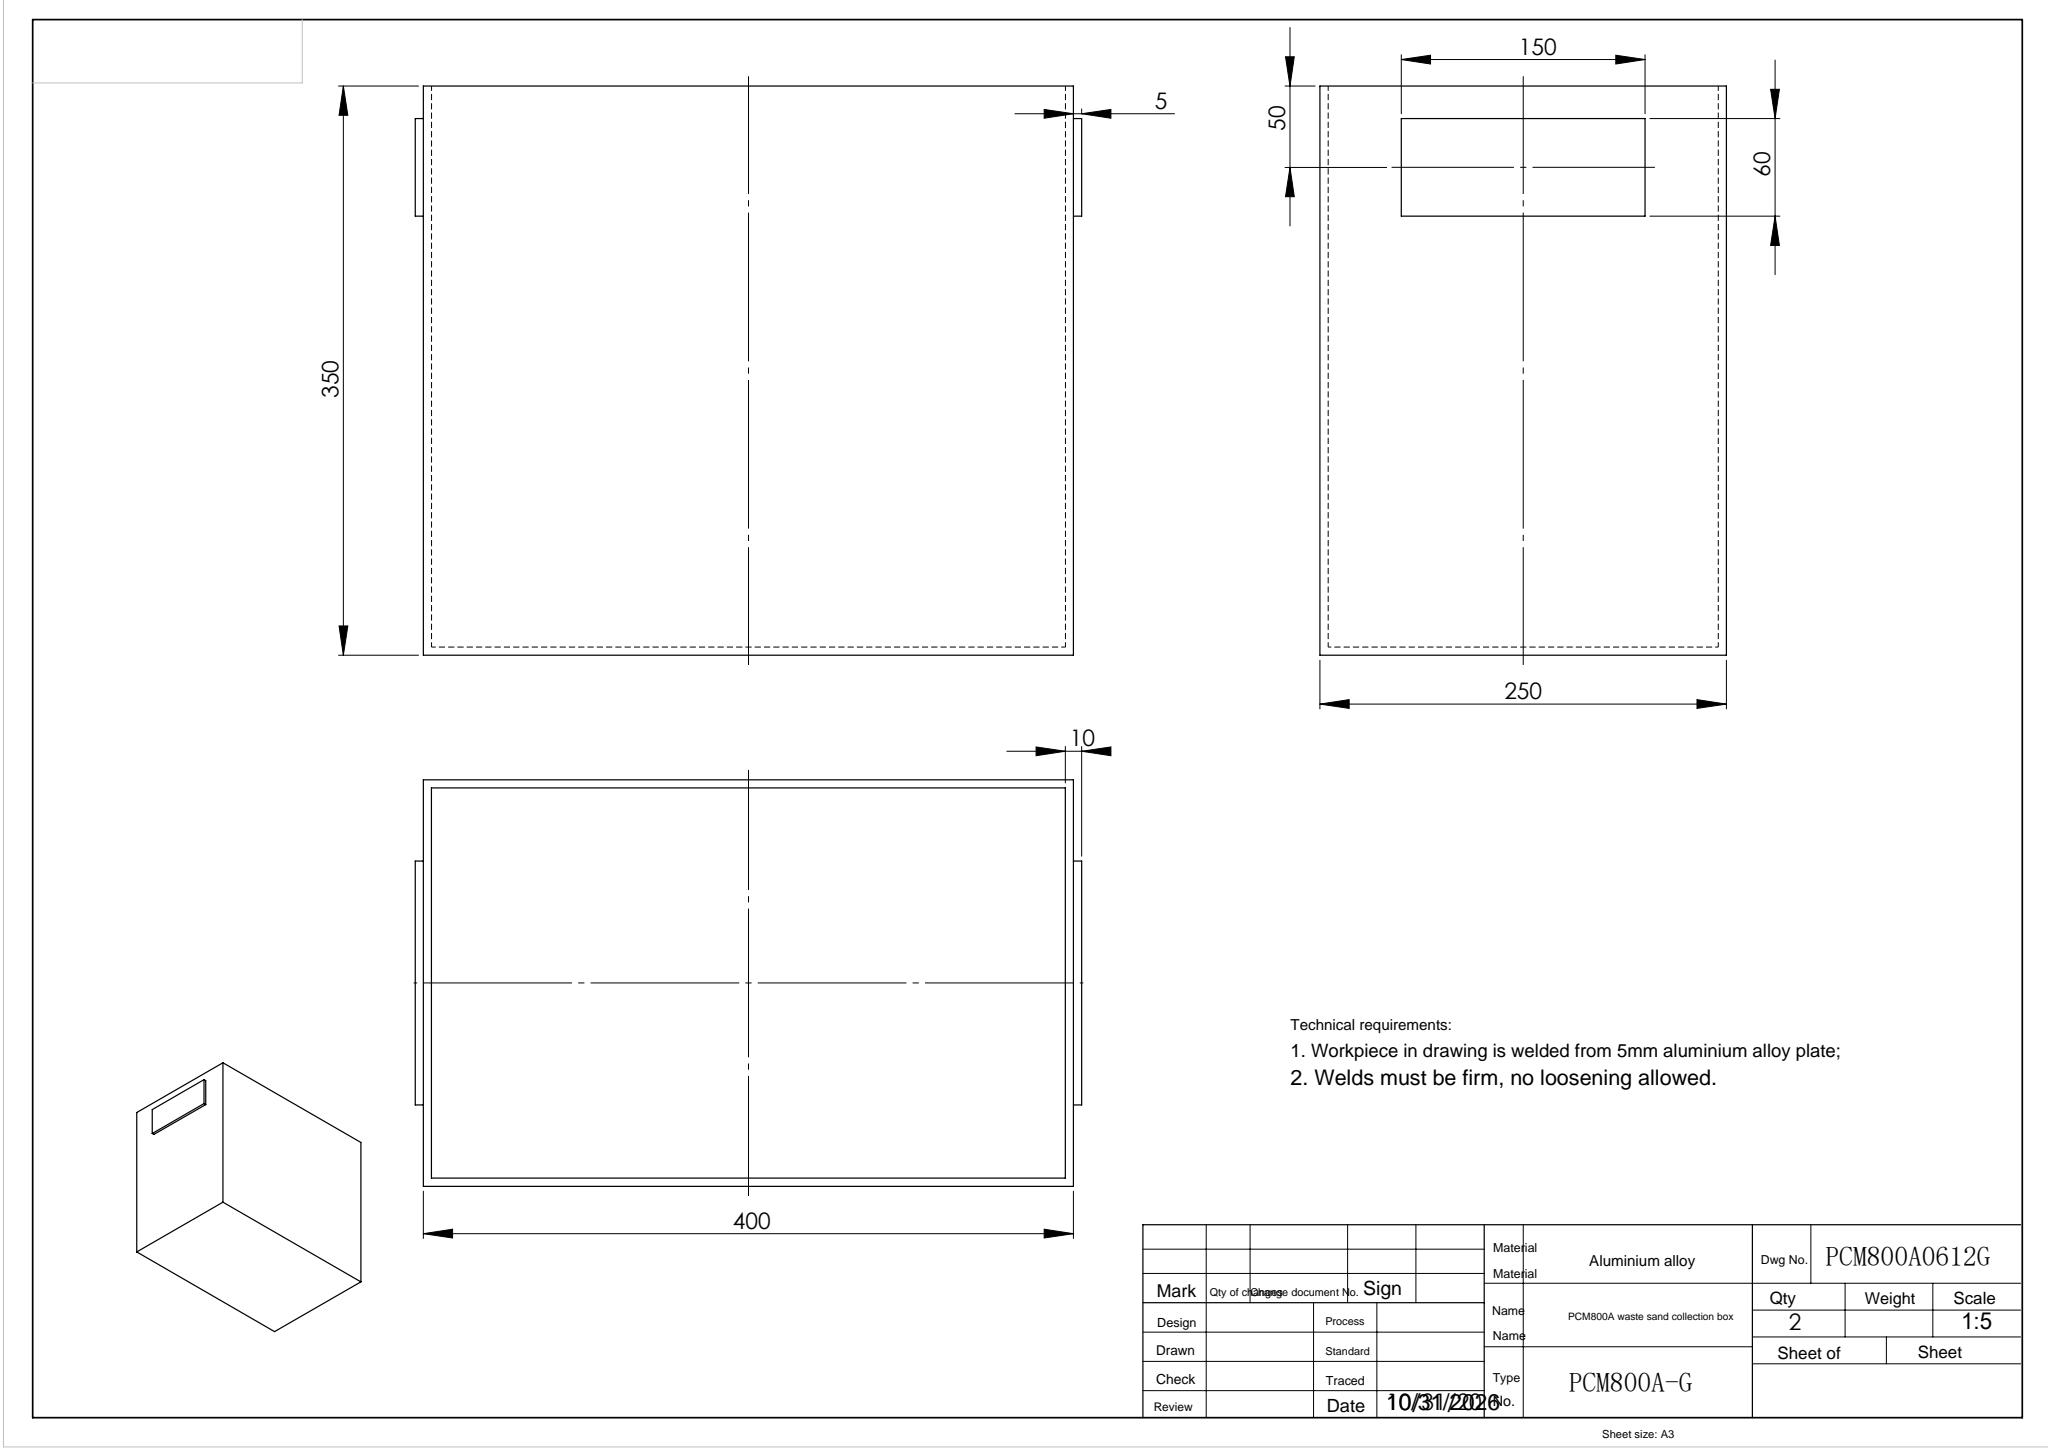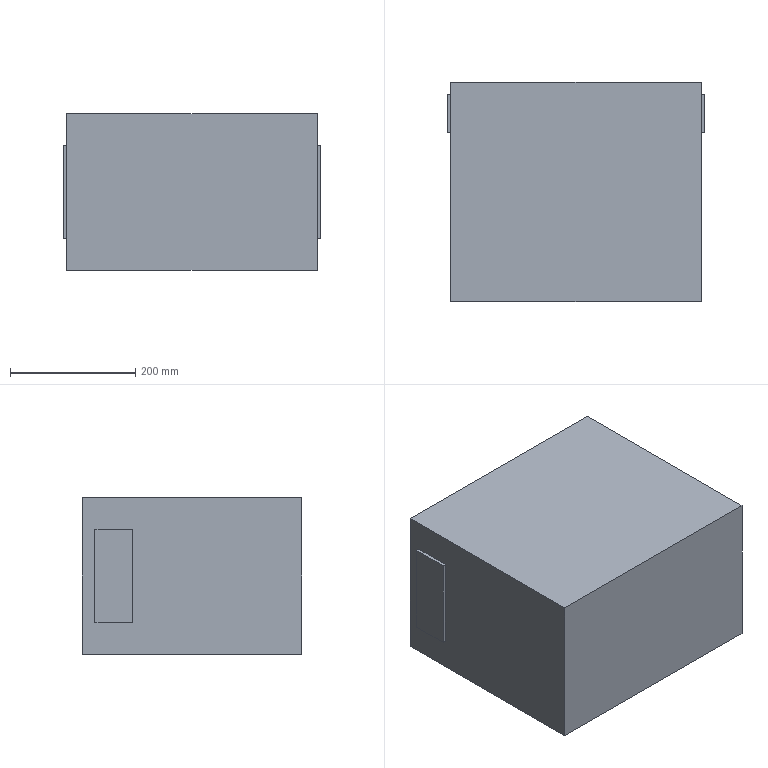Part | SolidWorks | features ICE 2, Extrusion 1, Shell 1 | 1 solid | 21 faces | box 410 x 350 x 250 mm | volume 2798000 mm3 | plane 21
STEP:
#1=CARTESIAN_POINT('',(0.,0.,-250.));
#2=VERTEX_POINT('',#1);
#3=CARTESIAN_POINT('',(0.,0.,0.));
#4=VERTEX_POINT('',#3);
#5=CARTESIAN_POINT('',(0.,0.,0.));
#6=DIRECTION('',(0.,0.,1.));
#7=VECTOR('',#6,1000.);
#8=LINE('',#5,#7);
#9=EDGE_CURVE('',#2,#4,#8,.T.);
#10=ORIENTED_EDGE('',*,*,#9,.T.);
#11=CARTESIAN_POINT('',(0.,350.,0.));
#12=VERTEX_POINT('',#11);
#13=CARTESIAN_POINT('',(0.,350.,0.));
#14=DIRECTION('',(0.,-1.,0.));
#15=VECTOR('',#14,1000.);
#16=LINE('',#13,#15);
#17=EDGE_CURVE('',#12,#4,#16,.T.);
#18=ORIENTED_EDGE('',*,*,#17,.F.);
#19=CARTESIAN_POINT('',(0.,350.,-250.));
#20=VERTEX_POINT('',#19);
#21=CARTESIAN_POINT('',(0.,350.,0.));
#22=DIRECTION('',(0.,0.,1.));
#23=VECTOR('',#22,1000.);
#24=LINE('',#21,#23);
#25=EDGE_CURVE('',#20,#12,#24,.T.);
#26=ORIENTED_EDGE('',*,*,#25,.F.);
#27=CARTESIAN_POINT('',(0.,350.,-250.));
#28=DIRECTION('',(0.,-1.,0.));
#29=VECTOR('',#28,1000.);
#30=LINE('',#27,#29);
#31=EDGE_CURVE('',#20,#2,#30,.T.);
#32=ORIENTED_EDGE('',*,*,#31,.T.);
#33=EDGE_LOOP('',(#10,#18,#26,#32));
#34=FACE_OUTER_BOUND('',#33,.T.);
#35=CARTESIAN_POINT('',(0.,330.,-200.));
#36=VERTEX_POINT('',#35);
#37=CARTESIAN_POINT('',(0.,270.,-200.));
#38=VERTEX_POINT('',#37);
#39=CARTESIAN_POINT('',(0.,330.,-200.));
#40=DIRECTION('',(0.,-1.,0.));
#41=VECTOR('',#40,1000.);
#42=LINE('',#39,#41);
#43=EDGE_CURVE('',#36,#38,#42,.T.);
#44=ORIENTED_EDGE('',*,*,#43,.F.);
#45=CARTESIAN_POINT('',(0.,330.,-50.));
#46=VERTEX_POINT('',#45);
#47=CARTESIAN_POINT('',(0.,330.,-200.));
#48=DIRECTION('',(0.,0.,-1.));
#49=VECTOR('',#48,1000.);
#50=LINE('',#47,#49);
#51=EDGE_CURVE('',#46,#36,#50,.T.);
#52=ORIENTED_EDGE('',*,*,#51,.F.);
#53=CARTESIAN_POINT('',(0.,270.,-50.));
#54=VERTEX_POINT('',#53);
#55=CARTESIAN_POINT('',(0.,330.,-50.));
#56=DIRECTION('',(0.,1.,0.));
#57=VECTOR('',#56,1000.);
#58=LINE('',#55,#57);
#59=EDGE_CURVE('',#54,#46,#58,.T.);
#60=ORIENTED_EDGE('',*,*,#59,.F.);
#61=CARTESIAN_POINT('',(0.,270.,-200.));
#62=DIRECTION('',(0.,0.,1.));
#63=VECTOR('',#62,1000.);
#64=LINE('',#61,#63);
#65=EDGE_CURVE('',#38,#54,#64,.T.);
#66=ORIENTED_EDGE('',*,*,#65,.F.);
#67=EDGE_LOOP('',(#44,#52,#60,#66));
#68=FACE_BOUND('',#67,.T.);
#69=CARTESIAN_POINT('',(0.,350.,0.));
#70=DIRECTION('',(1.,0.,0.));
#71=DIRECTION('',(0.,0.,-1.));
#72=AXIS2_PLACEMENT_3D('',#69,#70,#71);
#73=PLANE('',#72);
#74=ADVANCED_FACE('',(#34,#68),#73,.F.);
#75=CARTESIAN_POINT('',(400.,0.,0.));
#76=VERTEX_POINT('',#75);
#77=CARTESIAN_POINT('',(400.,0.,-250.));
#78=VERTEX_POINT('',#77);
#79=CARTESIAN_POINT('',(400.,0.,0.));
#80=DIRECTION('',(0.,0.,-1.));
#81=VECTOR('',#80,1000.);
#82=LINE('',#79,#81);
#83=EDGE_CURVE('',#76,#78,#82,.T.);
#84=ORIENTED_EDGE('',*,*,#83,.T.);
#85=CARTESIAN_POINT('',(400.,350.,-250.));
#86=VERTEX_POINT('',#85);
#87=CARTESIAN_POINT('',(400.,350.,-250.));
#88=DIRECTION('',(0.,-1.,0.));
#89=VECTOR('',#88,1000.);
#90=LINE('',#87,#89);
#91=EDGE_CURVE('',#86,#78,#90,.T.);
#92=ORIENTED_EDGE('',*,*,#91,.F.);
#93=CARTESIAN_POINT('',(400.,350.,0.));
#94=VERTEX_POINT('',#93);
#95=CARTESIAN_POINT('',(400.,350.,0.));
#96=DIRECTION('',(0.,0.,-1.));
#97=VECTOR('',#96,1000.);
#98=LINE('',#95,#97);
#99=EDGE_CURVE('',#94,#86,#98,.T.);
#100=ORIENTED_EDGE('',*,*,#99,.F.);
#101=CARTESIAN_POINT('',(400.,350.,0.));
#102=DIRECTION('',(0.,-1.,0.));
#103=VECTOR('',#102,1000.);
#104=LINE('',#101,#103);
#105=EDGE_CURVE('',#94,#76,#104,.T.);
#106=ORIENTED_EDGE('',*,*,#105,.T.);
#107=EDGE_LOOP('',(#84,#92,#100,#106));
#108=FACE_OUTER_BOUND('',#107,.T.);
#109=CARTESIAN_POINT('',(400.,330.,-50.));
#110=VERTEX_POINT('',#109);
#111=CARTESIAN_POINT('',(400.,270.,-50.));
#112=VERTEX_POINT('',#111);
#113=CARTESIAN_POINT('',(400.,330.,-50.));
#114=DIRECTION('',(0.,-1.,0.));
#115=VECTOR('',#114,1000.);
#116=LINE('',#113,#115);
#117=EDGE_CURVE('',#110,#112,#116,.T.);
#118=ORIENTED_EDGE('',*,*,#117,.F.);
#119=CARTESIAN_POINT('',(400.,330.,-200.));
#120=VERTEX_POINT('',#119);
#121=CARTESIAN_POINT('',(400.,330.,-50.));
#122=DIRECTION('',(0.,0.,1.));
#123=VECTOR('',#122,1000.);
#124=LINE('',#121,#123);
#125=EDGE_CURVE('',#120,#110,#124,.T.);
#126=ORIENTED_EDGE('',*,*,#125,.F.);
#127=CARTESIAN_POINT('',(400.,270.,-200.));
#128=VERTEX_POINT('',#127);
#129=CARTESIAN_POINT('',(400.,330.,-200.));
#130=DIRECTION('',(0.,1.,0.));
#131=VECTOR('',#130,1000.);
#132=LINE('',#129,#131);
#133=EDGE_CURVE('',#128,#120,#132,.T.);
#134=ORIENTED_EDGE('',*,*,#133,.F.);
#135=CARTESIAN_POINT('',(400.,270.,-50.));
#136=DIRECTION('',(0.,0.,-1.));
#137=VECTOR('',#136,1000.);
#138=LINE('',#135,#137);
#139=EDGE_CURVE('',#112,#128,#138,.T.);
#140=ORIENTED_EDGE('',*,*,#139,.F.);
#141=EDGE_LOOP('',(#118,#126,#134,#140));
#142=FACE_BOUND('',#141,.T.);
#143=CARTESIAN_POINT('',(400.,350.,0.));
#144=DIRECTION('',(-1.,0.,0.));
#145=DIRECTION('',(0.,0.,1.));
#146=AXIS2_PLACEMENT_3D('',#143,#144,#145);
#147=PLANE('',#146);
#148=ADVANCED_FACE('',(#108,#142),#147,.F.);
#149=ORIENTED_EDGE('',*,*,#25,.T.);
#150=CARTESIAN_POINT('',(0.,350.,0.));
#151=DIRECTION('',(1.,0.,0.));
#152=VECTOR('',#151,1000.);
#153=LINE('',#150,#152);
#154=EDGE_CURVE('',#12,#94,#153,.T.);
#155=ORIENTED_EDGE('',*,*,#154,.T.);
#156=ORIENTED_EDGE('',*,*,#99,.T.);
#157=CARTESIAN_POINT('',(0.,350.,-250.));
#158=DIRECTION('',(-1.,0.,0.));
#159=VECTOR('',#158,1000.);
#160=LINE('',#157,#159);
#161=EDGE_CURVE('',#86,#20,#160,.T.);
#162=ORIENTED_EDGE('',*,*,#161,.T.);
#163=EDGE_LOOP('',(#149,#155,#156,#162));
#164=FACE_OUTER_BOUND('',#163,.T.);
#165=CARTESIAN_POINT('',(5.,350.,-245.));
#166=VERTEX_POINT('',#165);
#167=CARTESIAN_POINT('',(5.,350.,-5.));
#168=VERTEX_POINT('',#167);
#169=CARTESIAN_POINT('',(5.,350.,-250.));
#170=DIRECTION('',(0.,0.,1.));
#171=VECTOR('',#170,1000.);
#172=LINE('',#169,#171);
#173=EDGE_CURVE('',#166,#168,#172,.T.);
#174=ORIENTED_EDGE('',*,*,#173,.F.);
#175=CARTESIAN_POINT('',(395.,350.,-245.));
#176=VERTEX_POINT('',#175);
#177=CARTESIAN_POINT('',(0.,350.,-245.));
#178=DIRECTION('',(-1.,0.,0.));
#179=VECTOR('',#178,1000.);
#180=LINE('',#177,#179);
#181=EDGE_CURVE('',#176,#166,#180,.T.);
#182=ORIENTED_EDGE('',*,*,#181,.F.);
#183=CARTESIAN_POINT('',(395.,350.,-5.));
#184=VERTEX_POINT('',#183);
#185=CARTESIAN_POINT('',(395.,350.,-250.));
#186=DIRECTION('',(0.,0.,-1.));
#187=VECTOR('',#186,1000.);
#188=LINE('',#185,#187);
#189=EDGE_CURVE('',#184,#176,#188,.T.);
#190=ORIENTED_EDGE('',*,*,#189,.F.);
#191=CARTESIAN_POINT('',(0.,350.,-5.));
#192=DIRECTION('',(1.,0.,0.));
#193=VECTOR('',#192,1000.);
#194=LINE('',#191,#193);
#195=EDGE_CURVE('',#168,#184,#194,.T.);
#196=ORIENTED_EDGE('',*,*,#195,.F.);
#197=EDGE_LOOP('',(#174,#182,#190,#196));
#198=FACE_BOUND('',#197,.T.);
#199=CARTESIAN_POINT('',(0.,350.,-250.));
#200=DIRECTION('',(0.,-1.,0.));
#201=DIRECTION('',(0.,0.,-1.));
#202=AXIS2_PLACEMENT_3D('',#199,#200,#201);
#203=PLANE('',#202);
#204=ADVANCED_FACE('',(#164,#198),#203,.F.);
#205=CARTESIAN_POINT('',(0.,0.,0.));
#206=DIRECTION('',(1.,0.,0.));
#207=VECTOR('',#206,1000.);
#208=LINE('',#205,#207);
#209=EDGE_CURVE('',#4,#76,#208,.T.);
#210=ORIENTED_EDGE('',*,*,#209,.T.);
#211=ORIENTED_EDGE('',*,*,#105,.F.);
#212=ORIENTED_EDGE('',*,*,#154,.F.);
#213=ORIENTED_EDGE('',*,*,#17,.T.);
#214=EDGE_LOOP('',(#210,#211,#212,#213));
#215=FACE_OUTER_BOUND('',#214,.T.);
#216=CARTESIAN_POINT('',(0.,350.,0.));
#217=DIRECTION('',(0.,0.,-1.));
#218=DIRECTION('',(-1.,0.,0.));
#219=AXIS2_PLACEMENT_3D('',#216,#217,#218);
#220=PLANE('',#219);
#221=ADVANCED_FACE('',(#215),#220,.F.);
#222=CARTESIAN_POINT('',(0.,0.,-250.));
#223=DIRECTION('',(-1.,0.,0.));
#224=VECTOR('',#223,1000.);
#225=LINE('',#222,#224);
#226=EDGE_CURVE('',#78,#2,#225,.T.);
#227=ORIENTED_EDGE('',*,*,#226,.T.);
#228=ORIENTED_EDGE('',*,*,#31,.F.);
#229=ORIENTED_EDGE('',*,*,#161,.F.);
#230=ORIENTED_EDGE('',*,*,#91,.T.);
#231=EDGE_LOOP('',(#227,#228,#229,#230));
#232=FACE_OUTER_BOUND('',#231,.T.);
#233=CARTESIAN_POINT('',(0.,350.,-250.));
#234=DIRECTION('',(0.,0.,1.));
#235=DIRECTION('',(1.,0.,0.));
#236=AXIS2_PLACEMENT_3D('',#233,#234,#235);
#237=PLANE('',#236);
#238=ADVANCED_FACE('',(#232),#237,.F.);
#239=ORIENTED_EDGE('',*,*,#9,.F.);
#240=ORIENTED_EDGE('',*,*,#226,.F.);
#241=ORIENTED_EDGE('',*,*,#83,.F.);
#242=ORIENTED_EDGE('',*,*,#209,.F.);
#243=EDGE_LOOP('',(#239,#240,#241,#242));
#244=FACE_OUTER_BOUND('',#243,.T.);
#245=CARTESIAN_POINT('',(0.,0.,-250.));
#246=DIRECTION('',(0.,-1.,0.));
#247=DIRECTION('',(0.,0.,-1.));
#248=AXIS2_PLACEMENT_3D('',#245,#246,#247);
#249=PLANE('',#248);
#250=ADVANCED_FACE('',(#244),#249,.T.);
#251=CARTESIAN_POINT('',(5.,5.,-245.));
#252=VERTEX_POINT('',#251);
#253=CARTESIAN_POINT('',(5.,5.,-5.));
#254=VERTEX_POINT('',#253);
#255=CARTESIAN_POINT('',(5.,5.,-250.));
#256=DIRECTION('',(0.,0.,1.));
#257=VECTOR('',#256,1000.);
#258=LINE('',#255,#257);
#259=EDGE_CURVE('',#252,#254,#258,.T.);
#260=ORIENTED_EDGE('',*,*,#259,.F.);
#261=CARTESIAN_POINT('',(5.,350.,-245.));
#262=DIRECTION('',(0.,-1.,0.));
#263=VECTOR('',#262,1000.);
#264=LINE('',#261,#263);
#265=EDGE_CURVE('',#166,#252,#264,.T.);
#266=ORIENTED_EDGE('',*,*,#265,.F.);
#267=ORIENTED_EDGE('',*,*,#173,.T.);
#268=CARTESIAN_POINT('',(5.,350.,-5.));
#269=DIRECTION('',(0.,-1.,0.));
#270=VECTOR('',#269,1000.);
#271=LINE('',#268,#270);
#272=EDGE_CURVE('',#168,#254,#271,.T.);
#273=ORIENTED_EDGE('',*,*,#272,.T.);
#274=EDGE_LOOP('',(#260,#266,#267,#273));
#275=FACE_OUTER_BOUND('',#274,.T.);
#276=CARTESIAN_POINT('',(5.,350.,0.));
#277=DIRECTION('',(1.,0.,0.));
#278=DIRECTION('',(0.,0.,-1.));
#279=AXIS2_PLACEMENT_3D('',#276,#277,#278);
#280=PLANE('',#279);
#281=ADVANCED_FACE('',(#275),#280,.T.);
#282=CARTESIAN_POINT('',(395.,5.,-5.));
#283=VERTEX_POINT('',#282);
#284=CARTESIAN_POINT('',(0.,5.,-5.));
#285=DIRECTION('',(1.,0.,0.));
#286=VECTOR('',#285,1000.);
#287=LINE('',#284,#286);
#288=EDGE_CURVE('',#254,#283,#287,.T.);
#289=ORIENTED_EDGE('',*,*,#288,.F.);
#290=ORIENTED_EDGE('',*,*,#272,.F.);
#291=ORIENTED_EDGE('',*,*,#195,.T.);
#292=CARTESIAN_POINT('',(395.,350.,-5.));
#293=DIRECTION('',(0.,-1.,0.));
#294=VECTOR('',#293,1000.);
#295=LINE('',#292,#294);
#296=EDGE_CURVE('',#184,#283,#295,.T.);
#297=ORIENTED_EDGE('',*,*,#296,.T.);
#298=EDGE_LOOP('',(#289,#290,#291,#297));
#299=FACE_OUTER_BOUND('',#298,.T.);
#300=CARTESIAN_POINT('',(0.,350.,-5.));
#301=DIRECTION('',(0.,0.,-1.));
#302=DIRECTION('',(-1.,0.,0.));
#303=AXIS2_PLACEMENT_3D('',#300,#301,#302);
#304=PLANE('',#303);
#305=ADVANCED_FACE('',(#299),#304,.T.);
#306=CARTESIAN_POINT('',(395.,5.,-245.));
#307=VERTEX_POINT('',#306);
#308=CARTESIAN_POINT('',(395.,5.,-250.));
#309=DIRECTION('',(0.,0.,-1.));
#310=VECTOR('',#309,1000.);
#311=LINE('',#308,#310);
#312=EDGE_CURVE('',#283,#307,#311,.T.);
#313=ORIENTED_EDGE('',*,*,#312,.F.);
#314=ORIENTED_EDGE('',*,*,#296,.F.);
#315=ORIENTED_EDGE('',*,*,#189,.T.);
#316=CARTESIAN_POINT('',(395.,350.,-245.));
#317=DIRECTION('',(0.,-1.,0.));
#318=VECTOR('',#317,1000.);
#319=LINE('',#316,#318);
#320=EDGE_CURVE('',#176,#307,#319,.T.);
#321=ORIENTED_EDGE('',*,*,#320,.T.);
#322=EDGE_LOOP('',(#313,#314,#315,#321));
#323=FACE_OUTER_BOUND('',#322,.T.);
#324=CARTESIAN_POINT('',(395.,350.,0.));
#325=DIRECTION('',(-1.,0.,0.));
#326=DIRECTION('',(0.,0.,1.));
#327=AXIS2_PLACEMENT_3D('',#324,#325,#326);
#328=PLANE('',#327);
#329=ADVANCED_FACE('',(#323),#328,.T.);
#330=CARTESIAN_POINT('',(0.,5.,-245.));
#331=DIRECTION('',(-1.,0.,0.));
#332=VECTOR('',#331,1000.);
#333=LINE('',#330,#332);
#334=EDGE_CURVE('',#307,#252,#333,.T.);
#335=ORIENTED_EDGE('',*,*,#334,.F.);
#336=ORIENTED_EDGE('',*,*,#320,.F.);
#337=ORIENTED_EDGE('',*,*,#181,.T.);
#338=ORIENTED_EDGE('',*,*,#265,.T.);
#339=EDGE_LOOP('',(#335,#336,#337,#338));
#340=FACE_OUTER_BOUND('',#339,.T.);
#341=CARTESIAN_POINT('',(0.,350.,-245.));
#342=DIRECTION('',(0.,0.,1.));
#343=DIRECTION('',(1.,0.,0.));
#344=AXIS2_PLACEMENT_3D('',#341,#342,#343);
#345=PLANE('',#344);
#346=ADVANCED_FACE('',(#340),#345,.T.);
#347=ORIENTED_EDGE('',*,*,#259,.T.);
#348=ORIENTED_EDGE('',*,*,#288,.T.);
#349=ORIENTED_EDGE('',*,*,#312,.T.);
#350=ORIENTED_EDGE('',*,*,#334,.T.);
#351=EDGE_LOOP('',(#347,#348,#349,#350));
#352=FACE_OUTER_BOUND('',#351,.T.);
#353=CARTESIAN_POINT('',(0.,5.,-250.));
#354=DIRECTION('',(0.,-1.,0.));
#355=DIRECTION('',(0.,0.,-1.));
#356=AXIS2_PLACEMENT_3D('',#353,#354,#355);
#357=PLANE('',#356);
#358=ADVANCED_FACE('',(#352),#357,.F.);
#359=ORIENTED_EDGE('',*,*,#117,.T.);
#360=CARTESIAN_POINT('',(405.,270.,-50.));
#361=VERTEX_POINT('',#360);
#362=CARTESIAN_POINT('',(405.,270.,-50.));
#363=DIRECTION('',(-1.,0.,0.));
#364=VECTOR('',#363,1000.);
#365=LINE('',#362,#364);
#366=EDGE_CURVE('',#361,#112,#365,.T.);
#367=ORIENTED_EDGE('',*,*,#366,.F.);
#368=CARTESIAN_POINT('',(405.,330.,-50.));
#369=VERTEX_POINT('',#368);
#370=CARTESIAN_POINT('',(405.,330.,-50.));
#371=DIRECTION('',(0.,-1.,0.));
#372=VECTOR('',#371,1000.);
#373=LINE('',#370,#372);
#374=EDGE_CURVE('',#369,#361,#373,.T.);
#375=ORIENTED_EDGE('',*,*,#374,.F.);
#376=CARTESIAN_POINT('',(405.,330.,-50.));
#377=DIRECTION('',(-1.,0.,0.));
#378=VECTOR('',#377,1000.);
#379=LINE('',#376,#378);
#380=EDGE_CURVE('',#369,#110,#379,.T.);
#381=ORIENTED_EDGE('',*,*,#380,.T.);
#382=EDGE_LOOP('',(#359,#367,#375,#381));
#383=FACE_OUTER_BOUND('',#382,.T.);
#384=CARTESIAN_POINT('',(405.,330.,-50.));
#385=DIRECTION('',(0.,0.,-1.));
#386=DIRECTION('',(0.,1.,0.));
#387=AXIS2_PLACEMENT_3D('',#384,#385,#386);
#388=PLANE('',#387);
#389=ADVANCED_FACE('',(#383),#388,.F.);
#390=ORIENTED_EDGE('',*,*,#139,.T.);
#391=CARTESIAN_POINT('',(405.,270.,-200.));
#392=VERTEX_POINT('',#391);
#393=CARTESIAN_POINT('',(405.,270.,-200.));
#394=DIRECTION('',(-1.,0.,0.));
#395=VECTOR('',#394,1000.);
#396=LINE('',#393,#395);
#397=EDGE_CURVE('',#392,#128,#396,.T.);
#398=ORIENTED_EDGE('',*,*,#397,.F.);
#399=CARTESIAN_POINT('',(405.,270.,-50.));
#400=DIRECTION('',(0.,0.,-1.));
#401=VECTOR('',#400,1000.);
#402=LINE('',#399,#401);
#403=EDGE_CURVE('',#361,#392,#402,.T.);
#404=ORIENTED_EDGE('',*,*,#403,.F.);
#405=ORIENTED_EDGE('',*,*,#366,.T.);
#406=EDGE_LOOP('',(#390,#398,#404,#405));
#407=FACE_OUTER_BOUND('',#406,.T.);
#408=CARTESIAN_POINT('',(405.,270.,-50.));
#409=DIRECTION('',(0.,1.,0.));
#410=DIRECTION('',(0.,0.,1.));
#411=AXIS2_PLACEMENT_3D('',#408,#409,#410);
#412=PLANE('',#411);
#413=ADVANCED_FACE('',(#407),#412,.F.);
#414=ORIENTED_EDGE('',*,*,#133,.T.);
#415=CARTESIAN_POINT('',(405.,330.,-200.));
#416=VERTEX_POINT('',#415);
#417=CARTESIAN_POINT('',(405.,330.,-200.));
#418=DIRECTION('',(-1.,0.,0.));
#419=VECTOR('',#418,1000.);
#420=LINE('',#417,#419);
#421=EDGE_CURVE('',#416,#120,#420,.T.);
#422=ORIENTED_EDGE('',*,*,#421,.F.);
#423=CARTESIAN_POINT('',(405.,330.,-200.));
#424=DIRECTION('',(0.,1.,0.));
#425=VECTOR('',#424,1000.);
#426=LINE('',#423,#425);
#427=EDGE_CURVE('',#392,#416,#426,.T.);
#428=ORIENTED_EDGE('',*,*,#427,.F.);
#429=ORIENTED_EDGE('',*,*,#397,.T.);
#430=EDGE_LOOP('',(#414,#422,#428,#429));
#431=FACE_OUTER_BOUND('',#430,.T.);
#432=CARTESIAN_POINT('',(405.,330.,-200.));
#433=DIRECTION('',(0.,0.,1.));
#434=DIRECTION('',(1.,0.,0.));
#435=AXIS2_PLACEMENT_3D('',#432,#433,#434);
#436=PLANE('',#435);
#437=ADVANCED_FACE('',(#431),#436,.F.);
#438=ORIENTED_EDGE('',*,*,#125,.T.);
#439=ORIENTED_EDGE('',*,*,#380,.F.);
#440=CARTESIAN_POINT('',(405.,330.,-50.));
#441=DIRECTION('',(0.,0.,1.));
#442=VECTOR('',#441,1000.);
#443=LINE('',#440,#442);
#444=EDGE_CURVE('',#416,#369,#443,.T.);
#445=ORIENTED_EDGE('',*,*,#444,.F.);
#446=ORIENTED_EDGE('',*,*,#421,.T.);
#447=EDGE_LOOP('',(#438,#439,#445,#446));
#448=FACE_OUTER_BOUND('',#447,.T.);
#449=CARTESIAN_POINT('',(405.,330.,-50.));
#450=DIRECTION('',(0.,-1.,0.));
#451=DIRECTION('',(0.,0.,-1.));
#452=AXIS2_PLACEMENT_3D('',#449,#450,#451);
#453=PLANE('',#452);
#454=ADVANCED_FACE('',(#448),#453,.F.);
#455=ORIENTED_EDGE('',*,*,#374,.T.);
#456=ORIENTED_EDGE('',*,*,#403,.T.);
#457=ORIENTED_EDGE('',*,*,#427,.T.);
#458=ORIENTED_EDGE('',*,*,#444,.T.);
#459=EDGE_LOOP('',(#455,#456,#457,#458));
#460=FACE_OUTER_BOUND('',#459,.T.);
#461=CARTESIAN_POINT('',(405.,270.,-50.));
#462=DIRECTION('',(1.,0.,0.));
#463=DIRECTION('',(0.,0.,-1.));
#464=AXIS2_PLACEMENT_3D('',#461,#462,#463);
#465=PLANE('',#464);
#466=ADVANCED_FACE('',(#460),#465,.T.);
#467=ORIENTED_EDGE('',*,*,#43,.T.);
#468=CARTESIAN_POINT('',(-5.,270.,-200.));
#469=VERTEX_POINT('',#468);
#470=CARTESIAN_POINT('',(-5.,270.,-200.));
#471=DIRECTION('',(1.,0.,0.));
#472=VECTOR('',#471,1000.);
#473=LINE('',#470,#472);
#474=EDGE_CURVE('',#469,#38,#473,.T.);
#475=ORIENTED_EDGE('',*,*,#474,.F.);
#476=CARTESIAN_POINT('',(-5.,330.,-200.));
#477=VERTEX_POINT('',#476);
#478=CARTESIAN_POINT('',(-5.,330.,-200.));
#479=DIRECTION('',(0.,-1.,0.));
#480=VECTOR('',#479,1000.);
#481=LINE('',#478,#480);
#482=EDGE_CURVE('',#477,#469,#481,.T.);
#483=ORIENTED_EDGE('',*,*,#482,.F.);
#484=CARTESIAN_POINT('',(-5.,330.,-200.));
#485=DIRECTION('',(1.,0.,0.));
#486=VECTOR('',#485,1000.);
#487=LINE('',#484,#486);
#488=EDGE_CURVE('',#477,#36,#487,.T.);
#489=ORIENTED_EDGE('',*,*,#488,.T.);
#490=EDGE_LOOP('',(#467,#475,#483,#489));
#491=FACE_OUTER_BOUND('',#490,.T.);
#492=CARTESIAN_POINT('',(-5.,330.,-200.));
#493=DIRECTION('',(0.,0.,1.));
#494=DIRECTION('',(0.,-1.,0.));
#495=AXIS2_PLACEMENT_3D('',#492,#493,#494);
#496=PLANE('',#495);
#497=ADVANCED_FACE('',(#491),#496,.F.);
#498=ORIENTED_EDGE('',*,*,#65,.T.);
#499=CARTESIAN_POINT('',(-5.,270.,-50.));
#500=VERTEX_POINT('',#499);
#501=CARTESIAN_POINT('',(-5.,270.,-50.));
#502=DIRECTION('',(1.,0.,0.));
#503=VECTOR('',#502,1000.);
#504=LINE('',#501,#503);
#505=EDGE_CURVE('',#500,#54,#504,.T.);
#506=ORIENTED_EDGE('',*,*,#505,.F.);
#507=CARTESIAN_POINT('',(-5.,270.,-200.));
#508=DIRECTION('',(0.,0.,1.));
#509=VECTOR('',#508,1000.);
#510=LINE('',#507,#509);
#511=EDGE_CURVE('',#469,#500,#510,.T.);
#512=ORIENTED_EDGE('',*,*,#511,.F.);
#513=ORIENTED_EDGE('',*,*,#474,.T.);
#514=EDGE_LOOP('',(#498,#506,#512,#513));
#515=FACE_OUTER_BOUND('',#514,.T.);
#516=CARTESIAN_POINT('',(-5.,270.,-200.));
#517=DIRECTION('',(0.,1.,0.));
#518=DIRECTION('',(0.,0.,1.));
#519=AXIS2_PLACEMENT_3D('',#516,#517,#518);
#520=PLANE('',#519);
#521=ADVANCED_FACE('',(#515),#520,.F.);
#522=ORIENTED_EDGE('',*,*,#59,.T.);
#523=CARTESIAN_POINT('',(-5.,330.,-50.));
#524=VERTEX_POINT('',#523);
#525=CARTESIAN_POINT('',(-5.,330.,-50.));
#526=DIRECTION('',(1.,0.,0.));
#527=VECTOR('',#526,1000.);
#528=LINE('',#525,#527);
#529=EDGE_CURVE('',#524,#46,#528,.T.);
#530=ORIENTED_EDGE('',*,*,#529,.F.);
#531=CARTESIAN_POINT('',(-5.,330.,-50.));
#532=DIRECTION('',(0.,1.,0.));
#533=VECTOR('',#532,1000.);
#534=LINE('',#531,#533);
#535=EDGE_CURVE('',#500,#524,#534,.T.);
#536=ORIENTED_EDGE('',*,*,#535,.F.);
#537=ORIENTED_EDGE('',*,*,#505,.T.);
#538=EDGE_LOOP('',(#522,#530,#536,#537));
#539=FACE_OUTER_BOUND('',#538,.T.);
#540=CARTESIAN_POINT('',(-5.,330.,-50.));
#541=DIRECTION('',(0.,0.,-1.));
#542=DIRECTION('',(0.,1.,0.));
#543=AXIS2_PLACEMENT_3D('',#540,#541,#542);
#544=PLANE('',#543);
#545=ADVANCED_FACE('',(#539),#544,.F.);
#546=ORIENTED_EDGE('',*,*,#51,.T.);
#547=ORIENTED_EDGE('',*,*,#488,.F.);
#548=CARTESIAN_POINT('',(-5.,330.,-200.));
#549=DIRECTION('',(0.,0.,-1.));
#550=VECTOR('',#549,1000.);
#551=LINE('',#548,#550);
#552=EDGE_CURVE('',#524,#477,#551,.T.);
#553=ORIENTED_EDGE('',*,*,#552,.F.);
#554=ORIENTED_EDGE('',*,*,#529,.T.);
#555=EDGE_LOOP('',(#546,#547,#553,#554));
#556=FACE_OUTER_BOUND('',#555,.T.);
#557=CARTESIAN_POINT('',(-5.,330.,-200.));
#558=DIRECTION('',(0.,-1.,0.));
#559=DIRECTION('',(0.,0.,-1.));
#560=AXIS2_PLACEMENT_3D('',#557,#558,#559);
#561=PLANE('',#560);
#562=ADVANCED_FACE('',(#556),#561,.F.);
#563=ORIENTED_EDGE('',*,*,#482,.T.);
#564=ORIENTED_EDGE('',*,*,#511,.T.);
#565=ORIENTED_EDGE('',*,*,#535,.T.);
#566=ORIENTED_EDGE('',*,*,#552,.T.);
#567=EDGE_LOOP('',(#563,#564,#565,#566));
#568=FACE_OUTER_BOUND('',#567,.T.);
#569=CARTESIAN_POINT('',(-5.,270.,-200.));
#570=DIRECTION('',(-1.,0.,0.));
#571=DIRECTION('',(0.,0.,1.));
#572=AXIS2_PLACEMENT_3D('',#569,#570,#571);
#573=PLANE('',#572);
#574=ADVANCED_FACE('',(#568),#573,.T.);
#575=CLOSED_SHELL('',(#74,#148,#204,#221,#238,#250,#281,#305,#329,#346,#358,#389,#413,#437,#454,#466,#497,#521,#545,#562,#574));
#576=MANIFOLD_SOLID_BREP('',#575);
#577=CARTESIAN_POINT('',(0.,0.,0.));
#578=DIRECTION('',(0.,0.,1.));
#579=DIRECTION('',(1.,0.,0.));
#580=AXIS2_PLACEMENT_3D('',#577,#578,#579);
#581=(LENGTH_UNIT()NAMED_UNIT(*)SI_UNIT(.MILLI.,.METRE.));
#582=UNCERTAINTY_MEASURE_WITH_UNIT(LENGTH_MEASURE(0.00001),#581,'','');
#583=(NAMED_UNIT(*)PLANE_ANGLE_UNIT()SI_UNIT($,.RADIAN.));
#584=(NAMED_UNIT(*)SI_UNIT($,.STERADIAN.)SOLID_ANGLE_UNIT());
#585=(GEOMETRIC_REPRESENTATION_CONTEXT(3)GLOBAL_UNCERTAINTY_ASSIGNED_CONTEXT((#582))GLOBAL_UNIT_ASSIGNED_CONTEXT((#581,#583,#584))REPRESENTATION_CONTEXT('',''));
#586=ADVANCED_BREP_SHAPE_REPRESENTATION('',(#576,#580),#585);